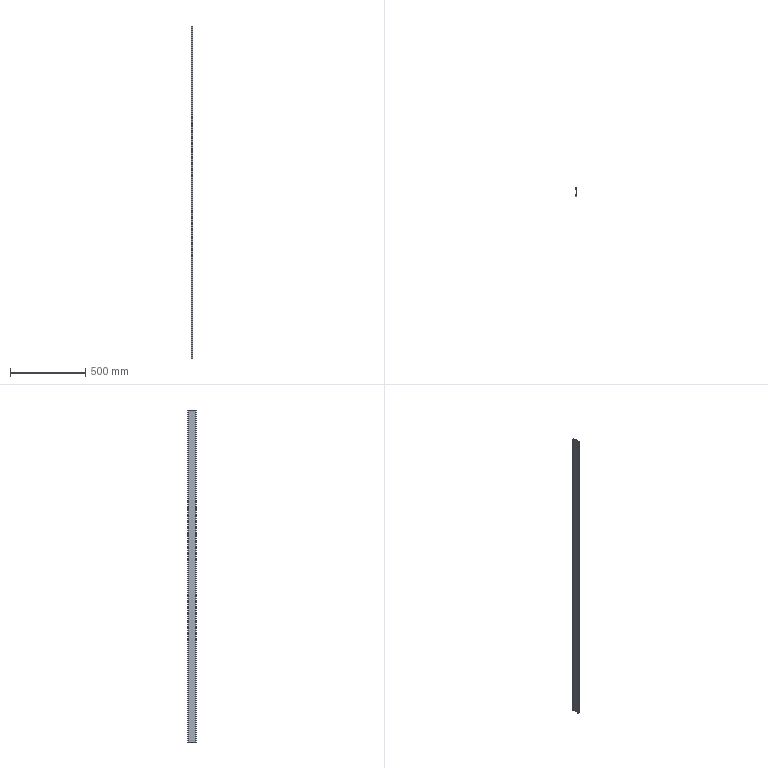Part | STEP file | Guide wheel mechanism revised.sldasm-Part-79 | 1 solid | 14 faces | box 12 x 56 x 2200 mm | volume 541200 mm3 | plane 14
STEP:
#1=CARTESIAN_POINT('',(3.,-25.,-1100.));
#2=VERTEX_POINT('',#1);
#3=CARTESIAN_POINT('',(-3.,-25.,-1100.));
#4=VERTEX_POINT('',#3);
#5=CARTESIAN_POINT('',(-3.,-25.,-1100.));
#6=DIRECTION('',(-1.,0.,0.));
#7=VECTOR('',#6,1000.);
#8=LINE('',#5,#7);
#9=EDGE_CURVE('',#2,#4,#8,.T.);
#10=ORIENTED_EDGE('',*,*,#9,.T.);
#11=CARTESIAN_POINT('',(-3.,-25.,1100.));
#12=VERTEX_POINT('',#11);
#13=CARTESIAN_POINT('',(-3.,-25.,1100.));
#14=DIRECTION('',(0.,0.,-1.));
#15=VECTOR('',#14,1000.);
#16=LINE('',#13,#15);
#17=EDGE_CURVE('',#12,#4,#16,.T.);
#18=ORIENTED_EDGE('',*,*,#17,.F.);
#19=CARTESIAN_POINT('',(3.,-25.,1100.));
#20=VERTEX_POINT('',#19);
#21=CARTESIAN_POINT('',(-3.,-25.,1100.));
#22=DIRECTION('',(-1.,0.,0.));
#23=VECTOR('',#22,1000.);
#24=LINE('',#21,#23);
#25=EDGE_CURVE('',#20,#12,#24,.T.);
#26=ORIENTED_EDGE('',*,*,#25,.F.);
#27=CARTESIAN_POINT('',(3.,-25.,1100.));
#28=DIRECTION('',(0.,0.,-1.));
#29=VECTOR('',#28,1000.);
#30=LINE('',#27,#29);
#31=EDGE_CURVE('',#20,#2,#30,.T.);
#32=ORIENTED_EDGE('',*,*,#31,.T.);
#33=EDGE_LOOP('',(#10,#18,#26,#32));
#34=FACE_OUTER_BOUND('',#33,.T.);
#35=CARTESIAN_POINT('',(-3.,-25.,1100.));
#36=DIRECTION('',(0.,-1.,0.));
#37=DIRECTION('',(0.,0.,-1.));
#38=AXIS2_PLACEMENT_3D('',#35,#36,#37);
#39=PLANE('',#38);
#40=ADVANCED_FACE('',(#34),#39,.F.);
#41=CARTESIAN_POINT('',(-3.,-21.,-1100.));
#42=VERTEX_POINT('',#41);
#43=CARTESIAN_POINT('',(-3.,-21.,-1100.));
#44=DIRECTION('',(0.,1.,0.));
#45=VECTOR('',#44,1000.);
#46=LINE('',#43,#45);
#47=EDGE_CURVE('',#4,#42,#46,.T.);
#48=ORIENTED_EDGE('',*,*,#47,.T.);
#49=CARTESIAN_POINT('',(-3.,-21.,1100.));
#50=VERTEX_POINT('',#49);
#51=CARTESIAN_POINT('',(-3.,-21.,1100.));
#52=DIRECTION('',(0.,0.,-1.));
#53=VECTOR('',#52,1000.);
#54=LINE('',#51,#53);
#55=EDGE_CURVE('',#50,#42,#54,.T.);
#56=ORIENTED_EDGE('',*,*,#55,.F.);
#57=CARTESIAN_POINT('',(-3.,-21.,1100.));
#58=DIRECTION('',(0.,1.,0.));
#59=VECTOR('',#58,1000.);
#60=LINE('',#57,#59);
#61=EDGE_CURVE('',#12,#50,#60,.T.);
#62=ORIENTED_EDGE('',*,*,#61,.F.);
#63=ORIENTED_EDGE('',*,*,#17,.T.);
#64=EDGE_LOOP('',(#48,#56,#62,#63));
#65=FACE_OUTER_BOUND('',#64,.T.);
#66=CARTESIAN_POINT('',(-3.,-21.,1100.));
#67=DIRECTION('',(-1.,0.,0.));
#68=DIRECTION('',(0.,0.,1.));
#69=AXIS2_PLACEMENT_3D('',#66,#67,#68);
#70=PLANE('',#69);
#71=ADVANCED_FACE('',(#65),#70,.F.);
#72=CARTESIAN_POINT('',(-6.,-21.,-1100.));
#73=VERTEX_POINT('',#72);
#74=CARTESIAN_POINT('',(-3.,-21.,-1100.));
#75=DIRECTION('',(-1.,0.,0.));
#76=VECTOR('',#75,1000.);
#77=LINE('',#74,#76);
#78=EDGE_CURVE('',#42,#73,#77,.T.);
#79=ORIENTED_EDGE('',*,*,#78,.T.);
#80=CARTESIAN_POINT('',(-6.,-21.,1100.));
#81=VERTEX_POINT('',#80);
#82=CARTESIAN_POINT('',(-6.,-21.,1100.));
#83=DIRECTION('',(0.,0.,-1.));
#84=VECTOR('',#83,1000.);
#85=LINE('',#82,#84);
#86=EDGE_CURVE('',#81,#73,#85,.T.);
#87=ORIENTED_EDGE('',*,*,#86,.F.);
#88=CARTESIAN_POINT('',(-3.,-21.,1100.));
#89=DIRECTION('',(-1.,0.,0.));
#90=VECTOR('',#89,1000.);
#91=LINE('',#88,#90);
#92=EDGE_CURVE('',#50,#81,#91,.T.);
#93=ORIENTED_EDGE('',*,*,#92,.F.);
#94=ORIENTED_EDGE('',*,*,#55,.T.);
#95=EDGE_LOOP('',(#79,#87,#93,#94));
#96=FACE_OUTER_BOUND('',#95,.T.);
#97=CARTESIAN_POINT('',(-3.,-21.,1100.));
#98=DIRECTION('',(0.,-1.,0.));
#99=DIRECTION('',(0.,0.,-1.));
#100=AXIS2_PLACEMENT_3D('',#97,#98,#99);
#101=PLANE('',#100);
#102=ADVANCED_FACE('',(#96),#101,.F.);
#103=CARTESIAN_POINT('',(-6.,-28.,-1100.));
#104=VERTEX_POINT('',#103);
#105=CARTESIAN_POINT('',(-6.,-21.,-1100.));
#106=DIRECTION('',(0.,-1.,0.));
#107=VECTOR('',#106,1000.);
#108=LINE('',#105,#107);
#109=EDGE_CURVE('',#73,#104,#108,.T.);
#110=ORIENTED_EDGE('',*,*,#109,.T.);
#111=CARTESIAN_POINT('',(-6.,-28.,1100.));
#112=VERTEX_POINT('',#111);
#113=CARTESIAN_POINT('',(-6.,-28.,1100.));
#114=DIRECTION('',(0.,0.,-1.));
#115=VECTOR('',#114,1000.);
#116=LINE('',#113,#115);
#117=EDGE_CURVE('',#112,#104,#116,.T.);
#118=ORIENTED_EDGE('',*,*,#117,.F.);
#119=CARTESIAN_POINT('',(-6.,-21.,1100.));
#120=DIRECTION('',(0.,-1.,0.));
#121=VECTOR('',#120,1000.);
#122=LINE('',#119,#121);
#123=EDGE_CURVE('',#81,#112,#122,.T.);
#124=ORIENTED_EDGE('',*,*,#123,.F.);
#125=ORIENTED_EDGE('',*,*,#86,.T.);
#126=EDGE_LOOP('',(#110,#118,#124,#125));
#127=FACE_OUTER_BOUND('',#126,.T.);
#128=CARTESIAN_POINT('',(-6.,-21.,1100.));
#129=DIRECTION('',(1.,0.,0.));
#130=DIRECTION('',(0.,0.,-1.));
#131=AXIS2_PLACEMENT_3D('',#128,#129,#130);
#132=PLANE('',#131);
#133=ADVANCED_FACE('',(#127),#132,.F.);
#134=CARTESIAN_POINT('',(6.,-28.,-1100.));
#135=VERTEX_POINT('',#134);
#136=CARTESIAN_POINT('',(-6.,-28.,-1100.));
#137=DIRECTION('',(1.,0.,0.));
#138=VECTOR('',#137,1000.);
#139=LINE('',#136,#138);
#140=EDGE_CURVE('',#104,#135,#139,.T.);
#141=ORIENTED_EDGE('',*,*,#140,.T.);
#142=CARTESIAN_POINT('',(6.,-28.,1100.));
#143=VERTEX_POINT('',#142);
#144=CARTESIAN_POINT('',(6.,-28.,1100.));
#145=DIRECTION('',(0.,0.,-1.));
#146=VECTOR('',#145,1000.);
#147=LINE('',#144,#146);
#148=EDGE_CURVE('',#143,#135,#147,.T.);
#149=ORIENTED_EDGE('',*,*,#148,.F.);
#150=CARTESIAN_POINT('',(-6.,-28.,1100.));
#151=DIRECTION('',(1.,0.,0.));
#152=VECTOR('',#151,1000.);
#153=LINE('',#150,#152);
#154=EDGE_CURVE('',#112,#143,#153,.T.);
#155=ORIENTED_EDGE('',*,*,#154,.F.);
#156=ORIENTED_EDGE('',*,*,#117,.T.);
#157=EDGE_LOOP('',(#141,#149,#155,#156));
#158=FACE_OUTER_BOUND('',#157,.T.);
#159=CARTESIAN_POINT('',(-6.,-28.,1100.));
#160=DIRECTION('',(0.,1.,0.));
#161=DIRECTION('',(0.,0.,1.));
#162=AXIS2_PLACEMENT_3D('',#159,#160,#161);
#163=PLANE('',#162);
#164=ADVANCED_FACE('',(#158),#163,.F.);
#165=CARTESIAN_POINT('',(6.,28.,-1100.));
#166=VERTEX_POINT('',#165);
#167=CARTESIAN_POINT('',(6.,-28.,-1100.));
#168=DIRECTION('',(0.,1.,0.));
#169=VECTOR('',#168,1000.);
#170=LINE('',#167,#169);
#171=EDGE_CURVE('',#135,#166,#170,.T.);
#172=ORIENTED_EDGE('',*,*,#171,.T.);
#173=CARTESIAN_POINT('',(6.,28.,1100.));
#174=VERTEX_POINT('',#173);
#175=CARTESIAN_POINT('',(6.,28.,1100.));
#176=DIRECTION('',(0.,0.,-1.));
#177=VECTOR('',#176,1000.);
#178=LINE('',#175,#177);
#179=EDGE_CURVE('',#174,#166,#178,.T.);
#180=ORIENTED_EDGE('',*,*,#179,.F.);
#181=CARTESIAN_POINT('',(6.,-28.,1100.));
#182=DIRECTION('',(0.,1.,0.));
#183=VECTOR('',#182,1000.);
#184=LINE('',#181,#183);
#185=EDGE_CURVE('',#143,#174,#184,.T.);
#186=ORIENTED_EDGE('',*,*,#185,.F.);
#187=ORIENTED_EDGE('',*,*,#148,.T.);
#188=EDGE_LOOP('',(#172,#180,#186,#187));
#189=FACE_OUTER_BOUND('',#188,.T.);
#190=CARTESIAN_POINT('',(6.,-28.,1100.));
#191=DIRECTION('',(-1.,0.,0.));
#192=DIRECTION('',(0.,0.,1.));
#193=AXIS2_PLACEMENT_3D('',#190,#191,#192);
#194=PLANE('',#193);
#195=ADVANCED_FACE('',(#189),#194,.F.);
#196=CARTESIAN_POINT('',(-6.,28.,-1100.));
#197=VERTEX_POINT('',#196);
#198=CARTESIAN_POINT('',(6.,28.,-1100.));
#199=DIRECTION('',(-1.,0.,0.));
#200=VECTOR('',#199,1000.);
#201=LINE('',#198,#200);
#202=EDGE_CURVE('',#166,#197,#201,.T.);
#203=ORIENTED_EDGE('',*,*,#202,.T.);
#204=CARTESIAN_POINT('',(-6.,28.,1100.));
#205=VERTEX_POINT('',#204);
#206=CARTESIAN_POINT('',(-6.,28.,1100.));
#207=DIRECTION('',(0.,0.,-1.));
#208=VECTOR('',#207,1000.);
#209=LINE('',#206,#208);
#210=EDGE_CURVE('',#205,#197,#209,.T.);
#211=ORIENTED_EDGE('',*,*,#210,.F.);
#212=CARTESIAN_POINT('',(6.,28.,1100.));
#213=DIRECTION('',(-1.,0.,0.));
#214=VECTOR('',#213,1000.);
#215=LINE('',#212,#214);
#216=EDGE_CURVE('',#174,#205,#215,.T.);
#217=ORIENTED_EDGE('',*,*,#216,.F.);
#218=ORIENTED_EDGE('',*,*,#179,.T.);
#219=EDGE_LOOP('',(#203,#211,#217,#218));
#220=FACE_OUTER_BOUND('',#219,.T.);
#221=CARTESIAN_POINT('',(6.,28.,1100.));
#222=DIRECTION('',(0.,-1.,0.));
#223=DIRECTION('',(1.,0.,0.));
#224=AXIS2_PLACEMENT_3D('',#221,#222,#223);
#225=PLANE('',#224);
#226=ADVANCED_FACE('',(#220),#225,.F.);
#227=CARTESIAN_POINT('',(-6.,21.,-1100.));
#228=VERTEX_POINT('',#227);
#229=CARTESIAN_POINT('',(-6.,28.,-1100.));
#230=DIRECTION('',(0.,-1.,0.));
#231=VECTOR('',#230,1000.);
#232=LINE('',#229,#231);
#233=EDGE_CURVE('',#197,#228,#232,.T.);
#234=ORIENTED_EDGE('',*,*,#233,.T.);
#235=CARTESIAN_POINT('',(-6.,21.,1100.));
#236=VERTEX_POINT('',#235);
#237=CARTESIAN_POINT('',(-6.,21.,1100.));
#238=DIRECTION('',(0.,0.,-1.));
#239=VECTOR('',#238,1000.);
#240=LINE('',#237,#239);
#241=EDGE_CURVE('',#236,#228,#240,.T.);
#242=ORIENTED_EDGE('',*,*,#241,.F.);
#243=CARTESIAN_POINT('',(-6.,28.,1100.));
#244=DIRECTION('',(0.,-1.,0.));
#245=VECTOR('',#244,1000.);
#246=LINE('',#243,#245);
#247=EDGE_CURVE('',#205,#236,#246,.T.);
#248=ORIENTED_EDGE('',*,*,#247,.F.);
#249=ORIENTED_EDGE('',*,*,#210,.T.);
#250=EDGE_LOOP('',(#234,#242,#248,#249));
#251=FACE_OUTER_BOUND('',#250,.T.);
#252=CARTESIAN_POINT('',(-6.,28.,1100.));
#253=DIRECTION('',(1.,0.,0.));
#254=DIRECTION('',(0.,1.,0.));
#255=AXIS2_PLACEMENT_3D('',#252,#253,#254);
#256=PLANE('',#255);
#257=ADVANCED_FACE('',(#251),#256,.F.);
#258=CARTESIAN_POINT('',(-3.,21.,-1100.));
#259=VERTEX_POINT('',#258);
#260=CARTESIAN_POINT('',(-3.,21.,-1100.));
#261=DIRECTION('',(1.,0.,0.));
#262=VECTOR('',#261,1000.);
#263=LINE('',#260,#262);
#264=EDGE_CURVE('',#228,#259,#263,.T.);
#265=ORIENTED_EDGE('',*,*,#264,.T.);
#266=CARTESIAN_POINT('',(-3.,21.,1100.));
#267=VERTEX_POINT('',#266);
#268=CARTESIAN_POINT('',(-3.,21.,1100.));
#269=DIRECTION('',(0.,0.,-1.));
#270=VECTOR('',#269,1000.);
#271=LINE('',#268,#270);
#272=EDGE_CURVE('',#267,#259,#271,.T.);
#273=ORIENTED_EDGE('',*,*,#272,.F.);
#274=CARTESIAN_POINT('',(-3.,21.,1100.));
#275=DIRECTION('',(1.,0.,0.));
#276=VECTOR('',#275,1000.);
#277=LINE('',#274,#276);
#278=EDGE_CURVE('',#236,#267,#277,.T.);
#279=ORIENTED_EDGE('',*,*,#278,.F.);
#280=ORIENTED_EDGE('',*,*,#241,.T.);
#281=EDGE_LOOP('',(#265,#273,#279,#280));
#282=FACE_OUTER_BOUND('',#281,.T.);
#283=CARTESIAN_POINT('',(-3.,21.,1100.));
#284=DIRECTION('',(0.,1.,0.));
#285=DIRECTION('',(0.,0.,1.));
#286=AXIS2_PLACEMENT_3D('',#283,#284,#285);
#287=PLANE('',#286);
#288=ADVANCED_FACE('',(#282),#287,.F.);
#289=CARTESIAN_POINT('',(-3.,25.,-1100.));
#290=VERTEX_POINT('',#289);
#291=CARTESIAN_POINT('',(-3.,25.,-1100.));
#292=DIRECTION('',(0.,1.,0.));
#293=VECTOR('',#292,1000.);
#294=LINE('',#291,#293);
#295=EDGE_CURVE('',#259,#290,#294,.T.);
#296=ORIENTED_EDGE('',*,*,#295,.T.);
#297=CARTESIAN_POINT('',(-3.,25.,1100.));
#298=VERTEX_POINT('',#297);
#299=CARTESIAN_POINT('',(-3.,25.,1100.));
#300=DIRECTION('',(0.,0.,-1.));
#301=VECTOR('',#300,1000.);
#302=LINE('',#299,#301);
#303=EDGE_CURVE('',#298,#290,#302,.T.);
#304=ORIENTED_EDGE('',*,*,#303,.F.);
#305=CARTESIAN_POINT('',(-3.,25.,1100.));
#306=DIRECTION('',(0.,1.,0.));
#307=VECTOR('',#306,1000.);
#308=LINE('',#305,#307);
#309=EDGE_CURVE('',#267,#298,#308,.T.);
#310=ORIENTED_EDGE('',*,*,#309,.F.);
#311=ORIENTED_EDGE('',*,*,#272,.T.);
#312=EDGE_LOOP('',(#296,#304,#310,#311));
#313=FACE_OUTER_BOUND('',#312,.T.);
#314=CARTESIAN_POINT('',(-3.,25.,1100.));
#315=DIRECTION('',(-1.,0.,0.));
#316=DIRECTION('',(0.,0.,1.));
#317=AXIS2_PLACEMENT_3D('',#314,#315,#316);
#318=PLANE('',#317);
#319=ADVANCED_FACE('',(#313),#318,.F.);
#320=CARTESIAN_POINT('',(3.,25.,-1100.));
#321=VERTEX_POINT('',#320);
#322=CARTESIAN_POINT('',(3.,25.,-1100.));
#323=DIRECTION('',(1.,0.,0.));
#324=VECTOR('',#323,1000.);
#325=LINE('',#322,#324);
#326=EDGE_CURVE('',#290,#321,#325,.T.);
#327=ORIENTED_EDGE('',*,*,#326,.T.);
#328=CARTESIAN_POINT('',(3.,25.,1100.));
#329=VERTEX_POINT('',#328);
#330=CARTESIAN_POINT('',(3.,25.,1100.));
#331=DIRECTION('',(0.,0.,-1.));
#332=VECTOR('',#331,1000.);
#333=LINE('',#330,#332);
#334=EDGE_CURVE('',#329,#321,#333,.T.);
#335=ORIENTED_EDGE('',*,*,#334,.F.);
#336=CARTESIAN_POINT('',(3.,25.,1100.));
#337=DIRECTION('',(1.,0.,0.));
#338=VECTOR('',#337,1000.);
#339=LINE('',#336,#338);
#340=EDGE_CURVE('',#298,#329,#339,.T.);
#341=ORIENTED_EDGE('',*,*,#340,.F.);
#342=ORIENTED_EDGE('',*,*,#303,.T.);
#343=EDGE_LOOP('',(#327,#335,#341,#342));
#344=FACE_OUTER_BOUND('',#343,.T.);
#345=CARTESIAN_POINT('',(3.,25.,1100.));
#346=DIRECTION('',(0.,1.,0.));
#347=DIRECTION('',(0.,0.,1.));
#348=AXIS2_PLACEMENT_3D('',#345,#346,#347);
#349=PLANE('',#348);
#350=ADVANCED_FACE('',(#344),#349,.F.);
#351=CARTESIAN_POINT('',(3.,-25.,-1100.));
#352=DIRECTION('',(0.,-1.,0.));
#353=VECTOR('',#352,1000.);
#354=LINE('',#351,#353);
#355=EDGE_CURVE('',#321,#2,#354,.T.);
#356=ORIENTED_EDGE('',*,*,#355,.T.);
#357=ORIENTED_EDGE('',*,*,#31,.F.);
#358=CARTESIAN_POINT('',(3.,-25.,1100.));
#359=DIRECTION('',(0.,-1.,0.));
#360=VECTOR('',#359,1000.);
#361=LINE('',#358,#360);
#362=EDGE_CURVE('',#329,#20,#361,.T.);
#363=ORIENTED_EDGE('',*,*,#362,.F.);
#364=ORIENTED_EDGE('',*,*,#334,.T.);
#365=EDGE_LOOP('',(#356,#357,#363,#364));
#366=FACE_OUTER_BOUND('',#365,.T.);
#367=CARTESIAN_POINT('',(3.,-25.,1100.));
#368=DIRECTION('',(1.,0.,0.));
#369=DIRECTION('',(0.,0.,-1.));
#370=AXIS2_PLACEMENT_3D('',#367,#368,#369);
#371=PLANE('',#370);
#372=ADVANCED_FACE('',(#366),#371,.F.);
#373=ORIENTED_EDGE('',*,*,#25,.T.);
#374=ORIENTED_EDGE('',*,*,#61,.T.);
#375=ORIENTED_EDGE('',*,*,#92,.T.);
#376=ORIENTED_EDGE('',*,*,#123,.T.);
#377=ORIENTED_EDGE('',*,*,#154,.T.);
#378=ORIENTED_EDGE('',*,*,#185,.T.);
#379=ORIENTED_EDGE('',*,*,#216,.T.);
#380=ORIENTED_EDGE('',*,*,#247,.T.);
#381=ORIENTED_EDGE('',*,*,#278,.T.);
#382=ORIENTED_EDGE('',*,*,#309,.T.);
#383=ORIENTED_EDGE('',*,*,#340,.T.);
#384=ORIENTED_EDGE('',*,*,#362,.T.);
#385=EDGE_LOOP('',(#373,#374,#375,#376,#377,#378,#379,#380,#381,#382,#383,#384));
#386=FACE_OUTER_BOUND('',#385,.T.);
#387=CARTESIAN_POINT('',(0.,0.,1100.));
#388=DIRECTION('',(0.,0.,1.));
#389=DIRECTION('',(1.,0.,0.));
#390=AXIS2_PLACEMENT_3D('',#387,#388,#389);
#391=PLANE('',#390);
#392=ADVANCED_FACE('',(#386),#391,.T.);
#393=ORIENTED_EDGE('',*,*,#9,.F.);
#394=ORIENTED_EDGE('',*,*,#355,.F.);
#395=ORIENTED_EDGE('',*,*,#326,.F.);
#396=ORIENTED_EDGE('',*,*,#295,.F.);
#397=ORIENTED_EDGE('',*,*,#264,.F.);
#398=ORIENTED_EDGE('',*,*,#233,.F.);
#399=ORIENTED_EDGE('',*,*,#202,.F.);
#400=ORIENTED_EDGE('',*,*,#171,.F.);
#401=ORIENTED_EDGE('',*,*,#140,.F.);
#402=ORIENTED_EDGE('',*,*,#109,.F.);
#403=ORIENTED_EDGE('',*,*,#78,.F.);
#404=ORIENTED_EDGE('',*,*,#47,.F.);
#405=EDGE_LOOP('',(#393,#394,#395,#396,#397,#398,#399,#400,#401,#402,#403,#404));
#406=FACE_OUTER_BOUND('',#405,.T.);
#407=CARTESIAN_POINT('',(0.,0.,-1100.));
#408=DIRECTION('',(0.,0.,1.));
#409=DIRECTION('',(1.,0.,0.));
#410=AXIS2_PLACEMENT_3D('',#407,#408,#409);
#411=PLANE('',#410);
#412=ADVANCED_FACE('',(#406),#411,.F.);
#413=CLOSED_SHELL('',(#40,#71,#102,#133,#164,#195,#226,#257,#288,#319,#350,#372,#392,#412));
#414=MANIFOLD_SOLID_BREP('',#413);
#415=CARTESIAN_POINT('',(0.,0.,0.));
#416=DIRECTION('',(0.,0.,1.));
#417=DIRECTION('',(1.,0.,0.));
#418=AXIS2_PLACEMENT_3D('',#415,#416,#417);
#419=(LENGTH_UNIT()NAMED_UNIT(*)SI_UNIT(.MILLI.,.METRE.));
#420=UNCERTAINTY_MEASURE_WITH_UNIT(LENGTH_MEASURE(0.00001),#419,'','');
#421=(NAMED_UNIT(*)PLANE_ANGLE_UNIT()SI_UNIT($,.RADIAN.));
#422=(NAMED_UNIT(*)SI_UNIT($,.STERADIAN.)SOLID_ANGLE_UNIT());
#423=(GEOMETRIC_REPRESENTATION_CONTEXT(3)GLOBAL_UNCERTAINTY_ASSIGNED_CONTEXT((#420))GLOBAL_UNIT_ASSIGNED_CONTEXT((#419,#421,#422))REPRESENTATION_CONTEXT('',''));
#424=ADVANCED_BREP_SHAPE_REPRESENTATION('',(#414,#418),#423);